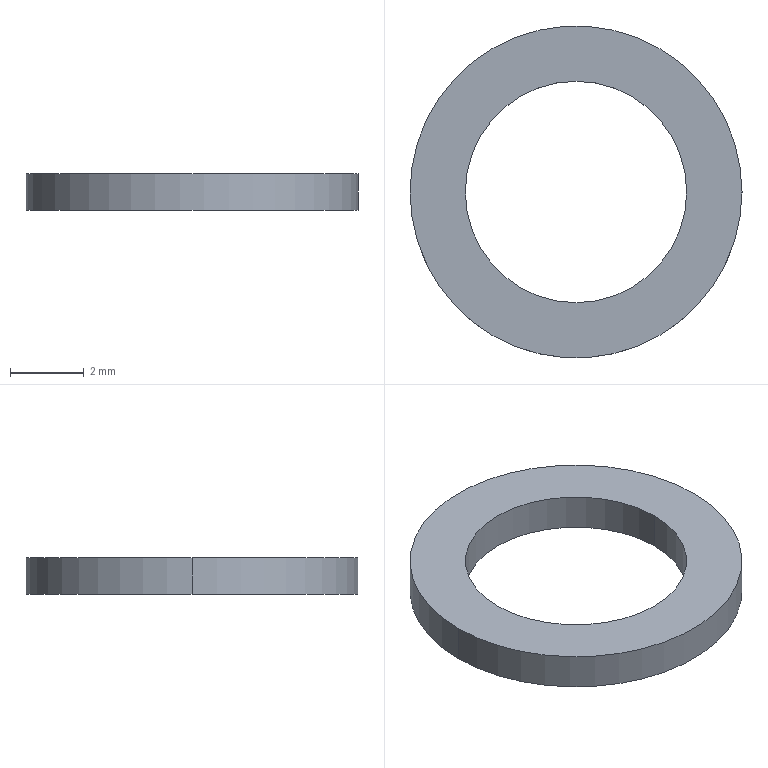Part | NX | features BREP 1 | 1 solid | 6 faces | box 9 x 9 x 1 mm | volume 35.343 mm3 | cylinder 4 | plane 2 | commonest cylinder face diameters 6 x2 9 x2
STEP:
#1=CARTESIAN_POINT('',(156.7,-545.367,1.));
#2=VERTEX_POINT('',#1);
#3=CARTESIAN_POINT('',(162.7,-545.367,1.));
#4=VERTEX_POINT('',#3);
#5=CARTESIAN_POINT('',(159.7,-545.367,1.));
#6=DIRECTION('',(0.,0.,1.));
#7=DIRECTION('',(1.,0.,0.));
#8=AXIS2_PLACEMENT_3D('',#5,#6,#7);
#9=CIRCLE('',#8,3.);
#10=EDGE_CURVE('',#2,#4,#9,.T.);
#11=ORIENTED_EDGE('',*,*,#10,.T.);
#12=CARTESIAN_POINT('',(162.7,-545.367,0.));
#13=VERTEX_POINT('',#12);
#14=CARTESIAN_POINT('',(162.7,-545.367,1.));
#15=DIRECTION('',(0.,0.,-1.));
#16=VECTOR('',#15,1000.);
#17=LINE('',#14,#16);
#18=EDGE_CURVE('',#13,#4,#17,.F.);
#19=ORIENTED_EDGE('',*,*,#18,.F.);
#20=CARTESIAN_POINT('',(156.7,-545.367,0.));
#21=VERTEX_POINT('',#20);
#22=CARTESIAN_POINT('',(159.7,-545.367,0.));
#23=DIRECTION('',(0.,0.,1.));
#24=DIRECTION('',(1.,0.,0.));
#25=AXIS2_PLACEMENT_3D('',#22,#23,#24);
#26=CIRCLE('',#25,3.);
#27=EDGE_CURVE('',#21,#13,#26,.T.);
#28=ORIENTED_EDGE('',*,*,#27,.F.);
#29=CARTESIAN_POINT('',(156.7,-545.367,1.));
#30=DIRECTION('',(0.,0.,-1.));
#31=VECTOR('',#30,1000.);
#32=LINE('',#29,#31);
#33=EDGE_CURVE('',#21,#2,#32,.F.);
#34=ORIENTED_EDGE('',*,*,#33,.T.);
#35=EDGE_LOOP('',(#11,#19,#28,#34));
#36=FACE_BOUND('',#35,.T.);
#37=CARTESIAN_POINT('',(159.7,-545.367,1.));
#38=DIRECTION('',(0.,0.,-1.));
#39=DIRECTION('',(1.,0.,0.));
#40=AXIS2_PLACEMENT_3D('',#37,#38,#39);
#41=CYLINDRICAL_SURFACE('',#40,3.);
#42=ADVANCED_FACE('',(#36),#41,.F.);
#43=CARTESIAN_POINT('',(164.2,-545.367,1.));
#44=VERTEX_POINT('',#43);
#45=CARTESIAN_POINT('',(155.2,-545.367,1.));
#46=VERTEX_POINT('',#45);
#47=CARTESIAN_POINT('',(159.7,-545.367,1.));
#48=DIRECTION('',(0.,0.,1.));
#49=DIRECTION('',(1.,0.,0.));
#50=AXIS2_PLACEMENT_3D('',#47,#48,#49);
#51=CIRCLE('',#50,4.5);
#52=EDGE_CURVE('',#44,#46,#51,.T.);
#53=ORIENTED_EDGE('',*,*,#52,.F.);
#54=CARTESIAN_POINT('',(164.2,-545.367,0.));
#55=VERTEX_POINT('',#54);
#56=CARTESIAN_POINT('',(164.2,-545.367,1.));
#57=DIRECTION('',(0.,0.,-1.));
#58=VECTOR('',#57,1000.);
#59=LINE('',#56,#58);
#60=EDGE_CURVE('',#55,#44,#59,.F.);
#61=ORIENTED_EDGE('',*,*,#60,.F.);
#62=CARTESIAN_POINT('',(155.2,-545.367,0.));
#63=VERTEX_POINT('',#62);
#64=CARTESIAN_POINT('',(159.7,-545.367,0.));
#65=DIRECTION('',(0.,0.,1.));
#66=DIRECTION('',(1.,0.,0.));
#67=AXIS2_PLACEMENT_3D('',#64,#65,#66);
#68=CIRCLE('',#67,4.5);
#69=EDGE_CURVE('',#55,#63,#68,.T.);
#70=ORIENTED_EDGE('',*,*,#69,.T.);
#71=CARTESIAN_POINT('',(155.2,-545.367,1.));
#72=DIRECTION('',(0.,0.,-1.));
#73=VECTOR('',#72,1000.);
#74=LINE('',#71,#73);
#75=EDGE_CURVE('',#63,#46,#74,.F.);
#76=ORIENTED_EDGE('',*,*,#75,.T.);
#77=EDGE_LOOP('',(#53,#61,#70,#76));
#78=FACE_BOUND('',#77,.T.);
#79=CARTESIAN_POINT('',(159.7,-545.367,1.));
#80=DIRECTION('',(0.,0.,-1.));
#81=DIRECTION('',(1.,0.,0.));
#82=AXIS2_PLACEMENT_3D('',#79,#80,#81);
#83=CYLINDRICAL_SURFACE('',#82,4.5);
#84=ADVANCED_FACE('',(#78),#83,.T.);
#85=CARTESIAN_POINT('',(159.7,-545.367,1.));
#86=DIRECTION('',(0.,0.,1.));
#87=DIRECTION('',(1.,0.,0.));
#88=AXIS2_PLACEMENT_3D('',#85,#86,#87);
#89=CIRCLE('',#88,4.5);
#90=EDGE_CURVE('',#46,#44,#89,.T.);
#91=ORIENTED_EDGE('',*,*,#90,.T.);
#92=ORIENTED_EDGE('',*,*,#52,.T.);
#93=EDGE_LOOP('',(#91,#92));
#94=FACE_BOUND('',#93,.T.);
#95=ORIENTED_EDGE('',*,*,#10,.F.);
#96=CARTESIAN_POINT('',(159.7,-545.367,1.));
#97=DIRECTION('',(0.,0.,1.));
#98=DIRECTION('',(1.,0.,0.));
#99=AXIS2_PLACEMENT_3D('',#96,#97,#98);
#100=CIRCLE('',#99,3.);
#101=EDGE_CURVE('',#4,#2,#100,.T.);
#102=ORIENTED_EDGE('',*,*,#101,.F.);
#103=EDGE_LOOP('',(#95,#102));
#104=FACE_BOUND('',#103,.T.);
#105=CARTESIAN_POINT('',(159.7,-545.367,1.));
#106=DIRECTION('',(0.,0.,1.));
#107=DIRECTION('',(-1.,0.,0.));
#108=AXIS2_PLACEMENT_3D('',#105,#106,#107);
#109=PLANE('',#108);
#110=ADVANCED_FACE('',(#94,#104),#109,.T.);
#111=CARTESIAN_POINT('',(159.7,-545.367,0.));
#112=DIRECTION('',(0.,0.,1.));
#113=DIRECTION('',(1.,0.,0.));
#114=AXIS2_PLACEMENT_3D('',#111,#112,#113);
#115=CIRCLE('',#114,4.5);
#116=EDGE_CURVE('',#63,#55,#115,.T.);
#117=ORIENTED_EDGE('',*,*,#116,.F.);
#118=ORIENTED_EDGE('',*,*,#69,.F.);
#119=EDGE_LOOP('',(#117,#118));
#120=FACE_BOUND('',#119,.T.);
#121=ORIENTED_EDGE('',*,*,#27,.T.);
#122=CARTESIAN_POINT('',(159.7,-545.367,0.));
#123=DIRECTION('',(0.,0.,1.));
#124=DIRECTION('',(1.,0.,0.));
#125=AXIS2_PLACEMENT_3D('',#122,#123,#124);
#126=CIRCLE('',#125,3.);
#127=EDGE_CURVE('',#13,#21,#126,.T.);
#128=ORIENTED_EDGE('',*,*,#127,.T.);
#129=EDGE_LOOP('',(#121,#128));
#130=FACE_BOUND('',#129,.T.);
#131=CARTESIAN_POINT('',(159.7,-545.367,0.));
#132=DIRECTION('',(0.,0.,1.));
#133=DIRECTION('',(-1.,0.,0.));
#134=AXIS2_PLACEMENT_3D('',#131,#132,#133);
#135=PLANE('',#134);
#136=ADVANCED_FACE('',(#120,#130),#135,.F.);
#137=ORIENTED_EDGE('',*,*,#60,.T.);
#138=ORIENTED_EDGE('',*,*,#90,.F.);
#139=ORIENTED_EDGE('',*,*,#75,.F.);
#140=ORIENTED_EDGE('',*,*,#116,.T.);
#141=EDGE_LOOP('',(#137,#138,#139,#140));
#142=FACE_BOUND('',#141,.T.);
#143=CARTESIAN_POINT('',(159.7,-545.367,1.));
#144=DIRECTION('',(0.,0.,-1.));
#145=DIRECTION('',(1.,0.,0.));
#146=AXIS2_PLACEMENT_3D('',#143,#144,#145);
#147=CYLINDRICAL_SURFACE('',#146,4.5);
#148=ADVANCED_FACE('',(#142),#147,.T.);
#149=ORIENTED_EDGE('',*,*,#18,.T.);
#150=ORIENTED_EDGE('',*,*,#101,.T.);
#151=ORIENTED_EDGE('',*,*,#33,.F.);
#152=ORIENTED_EDGE('',*,*,#127,.F.);
#153=EDGE_LOOP('',(#149,#150,#151,#152));
#154=FACE_BOUND('',#153,.T.);
#155=CARTESIAN_POINT('',(159.7,-545.367,1.));
#156=DIRECTION('',(0.,0.,-1.));
#157=DIRECTION('',(1.,0.,0.));
#158=AXIS2_PLACEMENT_3D('',#155,#156,#157);
#159=CYLINDRICAL_SURFACE('',#158,3.);
#160=ADVANCED_FACE('',(#154),#159,.F.);
#161=CLOSED_SHELL('',(#42,#84,#110,#136,#148,#160));
#162=MANIFOLD_SOLID_BREP('',#161);
#163=(LENGTH_UNIT()NAMED_UNIT(*)SI_UNIT(.MILLI.,.METRE.));
#164=UNCERTAINTY_MEASURE_WITH_UNIT(LENGTH_MEASURE(0.00001),#163,'','');
#165=(NAMED_UNIT(*)PLANE_ANGLE_UNIT()SI_UNIT($,.RADIAN.));
#166=(NAMED_UNIT(*)SI_UNIT($,.STERADIAN.)SOLID_ANGLE_UNIT());
#167=(GEOMETRIC_REPRESENTATION_CONTEXT(3)GLOBAL_UNCERTAINTY_ASSIGNED_CONTEXT((#164))GLOBAL_UNIT_ASSIGNED_CONTEXT((#163,#165,#166))REPRESENTATION_CONTEXT('',''));
#168=ADVANCED_BREP_SHAPE_REPRESENTATION('',(#162),#167);